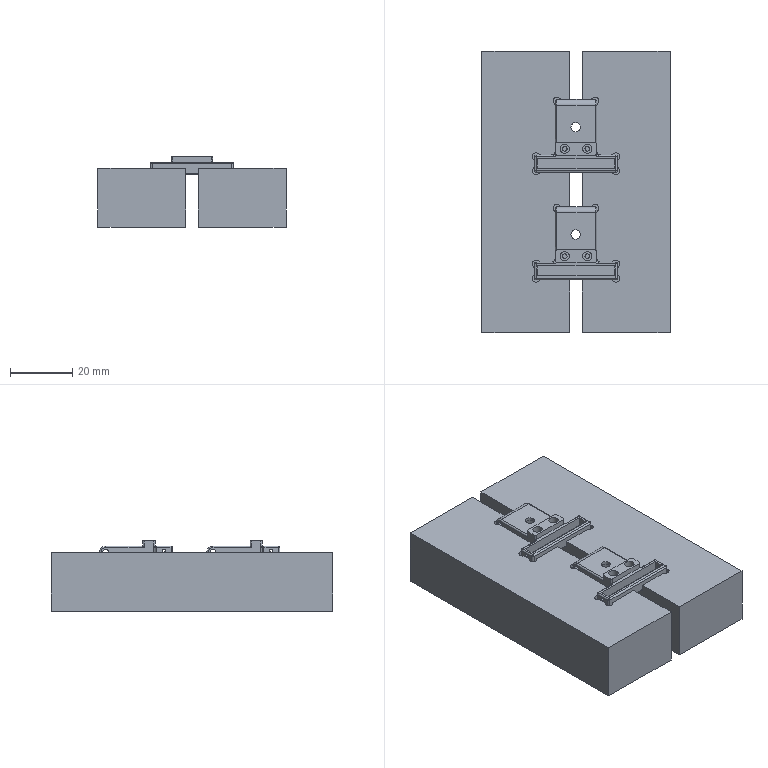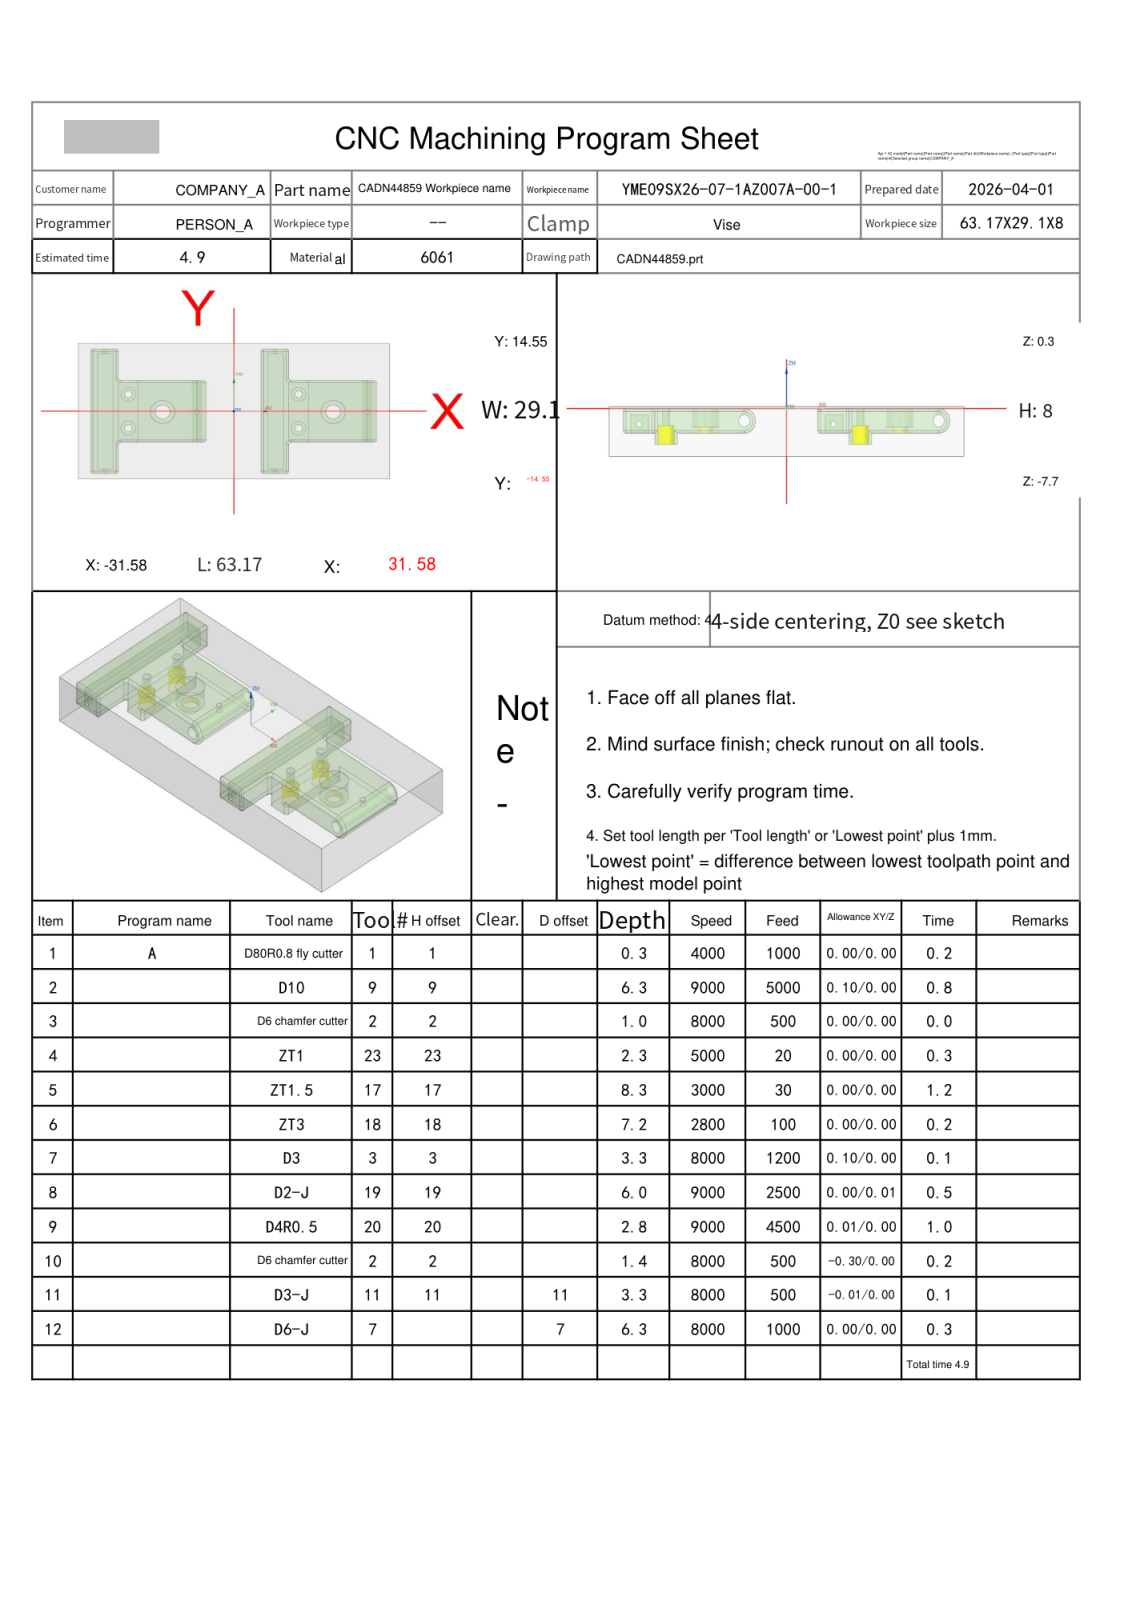NC program | NX | posted by the shop | part box 60.696 x 90.669 x 22.754 mm
Lines 834 to 2494 of 3978, first 1575 of 1661 lines:
N8 T19 M06
(D2-J  D=2. R=0. H=19 ce=0.00 di=0.01)
G00 G90 G54 X12.454 Y11.888 M03 S9000
G43 H19 Z20.
M08
Z.179
G01 X12.449 Y11.887 Z.124 F2000.
X12.435 Y11.884 Z.071
X12.414 Y11.879 Z.021
X12.386 Y11.871 Z-.027
X12.354 Y11.862 Z-.072
X12.319 Y11.849 Z-.113
X12.282 Y11.834 Z-.151
X12.245 Y11.817 Z-.185
X12.208 Y11.797 Z-.215
X12.174 Y11.774 Z-.24
X12.144 Y11.748 Z-.261
X12.12 Y11.719 Z-.276
X12.102 Y11.687 Z-.285
Y7.588 F2500.
X16.201
X16.215 Y7.603
X16.204 Y7.648 Z-.284
X16.17 Y7.719
X16.115 Y7.813 Z-.283
X15.9 Y8.13 Z-.284
X15.679 Y8.425 Z-.288
X15.384 Y8.799 Z-.299
X14.873 Y9.393 Z-.33
X14.412 Y9.885 Z-.369
X13.932 Y10.36 Z-.413
X13.348 Y10.887 Z-.468
X12.979 Y11.191 Z-.5
X12.687 Y11.419 Z-.526
X12.373 Y11.642 Z-.552
X12.279 Y11.7 Z-.56
X12.208 Y11.735 Z-.566
X12.163 Y11.747 Z-.569
X12.148 Y11.733 Z-.57
Y7.634
X16.247
X16.261 Y7.649 Z-.571
X16.25 Y7.694 Z-.574
X16.215 Y7.766 Z-.578
X16.159 Y7.861 Z-.583
X15.941 Y8.178 Z-.601
X15.718 Y8.473 Z-.619
X15.419 Y8.846 Z-.642
X14.902 Y9.435 Z-.68
X14.435 Y9.921 Z-.713
X13.949 Y10.388 Z-.746
X13.36 Y10.905 Z-.784
X12.987 Y11.204 Z-.807
X12.692 Y11.427 Z-.825
X12.375 Y11.646 Z-.843
X12.28 Y11.701 Z-.848
X12.208 Y11.736 Z-.852
X12.163 Y11.747 Z-.855
X12.148 Y11.733 Z-.856
Y7.634
X16.247
X16.261 Y7.649
X16.25 Y7.694 Z-.859
X16.215 Y7.766 Z-.863
X16.159 Y7.861 Z-.868
X15.941 Y8.178 Z-.887
X15.718 Y8.473 Z-.904
X15.419 Y8.846 Z-.927
X14.902 Y9.435 Z-.965
X14.435 Y9.921 Z-.998
X13.949 Y10.388 Z-1.031
X13.36 Y10.905 Z-1.07
X12.987 Y11.204 Z-1.092
X12.692 Y11.427 Z-1.11
X12.375 Y11.646 Z-1.128
X12.28 Y11.701 Z-1.133
X12.208 Y11.736 Z-1.137
X12.163 Y11.747 Z-1.14
X12.148 Y11.733 Z-1.141
Y7.634
X16.247
X16.261 Y7.649 Z-1.142
X16.25 Y7.694 Z-1.144
X16.215 Y7.766 Z-1.148
X16.159 Y7.861 Z-1.154
X15.941 Y8.178 Z-1.172
X15.718 Y8.473 Z-1.189
X15.419 Y8.846 Z-1.212
X14.902 Y9.435 Z-1.25
X14.435 Y9.921 Z-1.283
X13.949 Y10.388 Z-1.317
X13.36 Y10.905 Z-1.355
X12.987 Y11.204 Z-1.378
X12.692 Y11.427 Z-1.395
X12.375 Y11.646 Z-1.413
X12.28 Y11.701 Z-1.419
X12.208 Y11.736 Z-1.423
X12.163 Y11.747 Z-1.425
X12.148 Y11.733 Z-1.426
Y7.634
X16.247
X16.261 Y7.649 Z-1.427
X16.25 Y7.694 Z-1.429
X16.215 Y7.766 Z-1.433
X16.159 Y7.861 Z-1.439
X15.941 Y8.178 Z-1.457
X15.718 Y8.473 Z-1.475
X15.419 Y8.846 Z-1.497
X14.902 Y9.435 Z-1.535
X14.435 Y9.921 Z-1.569
X13.949 Y10.388 Z-1.602
X13.36 Y10.905 Z-1.64
X12.987 Y11.204 Z-1.663
X12.692 Y11.427 Z-1.68
X12.375 Y11.646 Z-1.698
X12.28 Y11.701 Z-1.704
X12.208 Y11.736 Z-1.708
X12.163 Y11.747 Z-1.71
X12.148 Y11.733 Z-1.711
Y7.634
X16.247
X16.261 Y7.649 Z-1.712
X16.25 Y7.694 Z-1.715
X16.215 Y7.766 Z-1.719
X16.159 Y7.861 Z-1.724
X15.941 Y8.178 Z-1.742
X15.718 Y8.473 Z-1.76
X15.419 Y8.846 Z-1.782
X14.902 Y9.435 Z-1.821
X14.435 Y9.921 Z-1.854
X13.949 Y10.388 Z-1.887
X13.36 Y10.905 Z-1.925
X12.987 Y11.204 Z-1.948
X12.692 Y11.427 Z-1.965
X12.375 Y11.646 Z-1.984
X12.28 Y11.701 Z-1.989
X12.208 Y11.736 Z-1.993
X12.163 Y11.747 Z-1.996
X12.148 Y11.733
Y7.634
X16.247
X16.261 Y7.649 Z-1.997
X16.25 Y7.694 Z-2.
X16.215 Y7.766 Z-2.004
X16.159 Y7.861 Z-2.009
X15.941 Y8.178 Z-2.027
X15.718 Y8.473 Z-2.045
X15.419 Y8.846 Z-2.068
X14.902 Y9.436 Z-2.106
X14.435 Y9.921 Z-2.139
X13.949 Y10.388 Z-2.172
X13.36 Y10.905 Z-2.21
X12.987 Y11.204 Z-2.233
X12.692 Y11.427 Z-2.251
X12.375 Y11.646 Z-2.269
X12.28 Y11.701 Z-2.274
X12.208 Y11.736 Z-2.278
X12.163 Y11.747 Z-2.281
X12.148 Y11.733 Z-2.282
Y7.634
X16.247
X16.261 Y7.649
X16.25 Y7.694 Z-2.285
X16.215 Y7.766 Z-2.289
X16.159 Y7.861 Z-2.294
X15.941 Y8.178 Z-2.313
X15.718 Y8.473 Z-2.33
X15.419 Y8.846 Z-2.353
X14.902 Y9.436 Z-2.391
X14.435 Y9.921 Z-2.424
X13.949 Y10.388 Z-2.457
X13.36 Y10.905 Z-2.496
X12.987 Y11.204 Z-2.518
X12.692 Y11.427 Z-2.536
X12.375 Y11.646 Z-2.554
X12.28 Y11.701 Z-2.559
X12.208 Y11.736 Z-2.563
X12.163 Y11.747 Z-2.566
X12.148 Y11.733 Z-2.567
Y7.634
X16.247
X16.261 Y7.649 Z-2.568
X16.25 Y7.694 Z-2.57
X16.215 Y7.766 Z-2.574
X16.159 Y7.861 Z-2.58
X15.941 Y8.178 Z-2.598
X15.718 Y8.473 Z-2.615
X15.419 Y8.846 Z-2.638
X14.902 Y9.436 Z-2.676
X14.435 Y9.921 Z-2.709
X13.949 Y10.388 Z-2.743
X13.36 Y10.905 Z-2.781
X12.987 Y11.204 Z-2.804
X12.692 Y11.427 Z-2.821
X12.375 Y11.646 Z-2.839
X12.28 Y11.701 Z-2.845
X12.208 Y11.736 Z-2.849
X12.163 Y11.747 Z-2.851
X12.148 Y11.733 Z-2.852
Y7.634
X16.247
X16.261 Y7.649 Z-2.853
X16.25 Y7.694 Z-2.855
X16.215 Y7.766 Z-2.859
X16.159 Y7.861 Z-2.865
X15.941 Y8.178 Z-2.883
X15.718 Y8.473 Z-2.901
X15.419 Y8.846 Z-2.923
X14.902 Y9.436 Z-2.961
X14.435 Y9.921 Z-2.995
X13.949 Y10.388 Z-3.028
X13.36 Y10.905 Z-3.066
X12.987 Y11.204 Z-3.089
X12.692 Y11.427 Z-3.106
X12.375 Y11.646 Z-3.125
X12.28 Y11.701 Z-3.13
X12.208 Y11.736 Z-3.134
X12.163 Y11.747 Z-3.136
X12.148 Y11.733 Z-3.137
Y7.634
X16.247
X16.261 Y7.649 Z-3.138
X16.25 Y7.694 Z-3.141
X16.215 Y7.766 Z-3.145
X16.159 Y7.861 Z-3.15
X15.941 Y8.178 Z-3.168
X15.718 Y8.473 Z-3.186
X15.419 Y8.846 Z-3.208
X14.902 Y9.436 Z-3.247
X14.435 Y9.921 Z-3.28
X13.949 Y10.388 Z-3.313
X13.36 Y10.905 Z-3.351
X12.987 Y11.204 Z-3.374
X12.692 Y11.427 Z-3.391
X12.375 Y11.646 Z-3.41
X12.28 Y11.701 Z-3.415
X12.208 Y11.736 Z-3.419
X12.163 Y11.747 Z-3.422
X12.148 Y11.733
Y7.634
X16.247
X16.261 Y7.649 Z-3.423
X16.25 Y7.694 Z-3.426
X16.215 Y7.766 Z-3.43
X16.159 Y7.861 Z-3.435
X15.941 Y8.178 Z-3.453
X15.718 Y8.474 Z-3.471
X15.419 Y8.847 Z-3.494
X14.902 Y9.437 Z-3.532
X14.435 Y9.923 Z-3.565
X13.949 Y10.39 Z-3.598
X13.36 Y10.907 Z-3.636
X12.987 Y11.207 Z-3.659
X12.692 Y11.43 Z-3.677
X12.375 Y11.649 Z-3.695
X12.28 Y11.705 Z-3.7
X12.208 Y11.739 Z-3.704
X12.163 Y11.751 Z-3.707
X12.148 Y11.737 Z-3.708
Y7.634
X16.249
X16.263 Y7.649
X16.252 Y7.694 Z-3.711
X16.217 Y7.766 Z-3.715
X16.161 Y7.861 Z-3.72
X15.943 Y8.178 Z-3.739
X15.72 Y8.474 Z-3.756
X15.42 Y8.847 Z-3.779
X14.903 Y9.437 Z-3.817
X14.436 Y9.923 Z-3.85
X13.95 Y10.39 Z-3.883
X13.36 Y10.907 Z-3.922
X12.987 Y11.207 Z-3.944
X12.692 Y11.43 Z-3.962
X12.375 Y11.649 Z-3.98
X12.28 Y11.705 Z-3.985
X12.208 Y11.739 Z-3.989
X12.163 Y11.751 Z-3.992
X12.148 Y11.737 Z-3.993
Y7.634
X16.249
X16.263 Y7.649 Z-3.994
X16.252 Y7.694 Z-3.996
X16.217 Y7.766 Z-4.
X16.161 Y7.861 Z-4.006
X15.943 Y8.178 Z-4.024
X15.72 Y8.474 Z-4.041
X15.42 Y8.847 Z-4.064
X14.903 Y9.437 Z-4.102
X14.436 Y9.923 Z-4.135
X13.95 Y10.39 Z-4.169
X13.36 Y10.907 Z-4.207
X12.987 Y11.207 Z-4.23
X12.692 Y11.43 Z-4.247
X12.375 Y11.649 Z-4.265
X12.28 Y11.705 Z-4.271
X12.208 Y11.739 Z-4.275
X12.163 Y11.751 Z-4.277
X12.148 Y11.737 Z-4.278
Y7.634
X16.249
X16.263 Y7.649 Z-4.279
X16.252 Y7.694 Z-4.281
X16.217 Y7.766 Z-4.285
X16.161 Y7.861 Z-4.291
X15.943 Y8.178 Z-4.309
X15.72 Y8.474 Z-4.327
X15.42 Y8.847 Z-4.349
X14.903 Y9.437 Z-4.387
X14.436 Y9.923 Z-4.421
X13.95 Y10.39 Z-4.454
X13.36 Y10.907 Z-4.492
X12.987 Y11.207 Z-4.515
X12.692 Y11.43 Z-4.532
X12.375 Y11.649 Z-4.551
X12.28 Y11.705 Z-4.556
X12.208 Y11.739 Z-4.56
X12.163 Y11.751 Z-4.562
X12.148 Y11.737 Z-4.563
Y7.634
X16.249
X16.263 Y7.649 Z-4.564
X16.252 Y7.694 Z-4.567
X16.217 Y7.766 Z-4.571
X16.161 Y7.861 Z-4.576
X15.943 Y8.178 Z-4.594
X15.72 Y8.474 Z-4.612
X15.42 Y8.847 Z-4.634
X14.903 Y9.437 Z-4.673
X14.436 Y9.923 Z-4.706
X13.95 Y10.39 Z-4.739
X13.36 Y10.907 Z-4.777
X12.987 Y11.207 Z-4.8
X12.692 Y11.43 Z-4.817
X12.375 Y11.649 Z-4.836
X12.28 Y11.705 Z-4.841
X12.208 Y11.739 Z-4.845
X12.163 Y11.751 Z-4.848
X12.148 Y11.737
Y7.634
X16.249
X16.263 Y7.649 Z-4.849
X16.252 Y7.694 Z-4.852
X16.217 Y7.766 Z-4.856
X16.161 Y7.861 Z-4.861
X15.943 Y8.178 Z-4.879
X15.72 Y8.474 Z-4.897
X15.42 Y8.847 Z-4.92
X14.903 Y9.437 Z-4.958
X14.436 Y9.923 Z-4.991
X13.95 Y10.39 Z-5.024
X13.36 Y10.907 Z-5.062
X12.987 Y11.207 Z-5.085
X12.692 Y11.43 Z-5.103
X12.375 Y11.649 Z-5.121
X12.28 Y11.705 Z-5.126
X12.208 Y11.739 Z-5.13
X12.163 Y11.751 Z-5.133
X12.148 Y11.737 Z-5.134
Y7.634
X16.249
X16.263 Y7.649
X16.252 Y7.694 Z-5.137
X16.217 Y7.766 Z-5.141
X16.161 Y7.861 Z-5.146
X15.943 Y8.178 Z-5.165
X15.72 Y8.474 Z-5.182
X15.42 Y8.847 Z-5.205
X14.903 Y9.437 Z-5.243
X14.436 Y9.923 Z-5.276
X13.95 Y10.39 Z-5.309
X13.36 Y10.907 Z-5.348
X12.987 Y11.207 Z-5.37
X12.692 Y11.43 Z-5.388
X12.375 Y11.649 Z-5.406
X12.28 Y11.705 Z-5.411
X12.208 Y11.739 Z-5.415
X12.163 Y11.751 Z-5.418
X12.148 Y11.737 Z-5.419
Y7.634
X16.249
X16.263 Y7.649 Z-5.42
X16.252 Y7.694 Z-5.422
X16.217 Y7.766 Z-5.426
X16.161 Y7.861 Z-5.432
X15.943 Y8.178 Z-5.45
X15.72 Y8.474 Z-5.467
X15.42 Y8.847 Z-5.49
X14.903 Y9.437 Z-5.528
X14.436 Y9.923 Z-5.561
X13.95 Y10.39 Z-5.595
X13.36 Y10.907 Z-5.633
X12.987 Y11.207 Z-5.656
X12.692 Y11.43 Z-5.673
X12.375 Y11.649 Z-5.691
X12.28 Y11.705 Z-5.697
X12.208 Y11.739 Z-5.701
X12.163 Y11.751 Z-5.703
X12.148 Y11.737 Z-5.704
Y7.634
X16.249
X16.363 Y7.643 Z-5.702
X16.466 Y7.67 Z-5.695
X16.558 Y7.712 Z-5.684
X16.639 Y7.765 Z-5.666
X16.71 Y7.828 Z-5.643
X16.772 Y7.898 Z-5.613
X16.826 Y7.972 Z-5.576
X16.871 Y8.047 Z-5.531
X16.908 Y8.12 Z-5.477
X16.938 Y8.19 Z-5.415
X16.961 Y8.253 Z-5.344
X16.979 Y8.306 Z-5.262
X16.99 Y8.348 Z-5.171
X16.997 Y8.375 Z-5.068
X16.999 Y8.384 Z-4.954
G00 Z20.
X16.382 Y-7.937
Z.176
G01 Y-7.932 Z.122 F2000.
X16.379 Y-7.918 Z.069
X16.376 Y-7.897 Z.019
X16.37 Y-7.87 Z-.029
X16.362 Y-7.838 Z-.073
X16.352 Y-7.803 Z-.115
X16.339 Y-7.767 Z-.152
X16.324 Y-7.73 Z-.186
X16.306 Y-7.694 Z-.216
X16.285 Y-7.66 Z-.241
X16.261 Y-7.63 Z-.261
X16.233 Y-7.606 Z-.276
X16.201 Y-7.588 Z-.285
X12.102 F2500.
Y-11.687
X12.117 Y-11.701
X12.162 Y-11.69 Z-.284
X12.233 Y-11.657
X12.327 Y-11.602 Z-.283
X12.644 Y-11.387 Z-.284
X12.939 Y-11.167 Z-.288
X13.313 Y-10.872 Z-.298
X13.907 Y-10.362 Z-.33
X14.399 Y-9.901 Z-.369
X14.874 Y-9.421 Z-.413
X15.401 Y-8.837 Z-.467
X15.705 Y-8.468 Z-.5
X15.933 Y-8.174 Z-.526
X16.156 Y-7.859 Z-.552
X16.213 Y-7.765 Z-.56
X16.249 Y-7.694 Z-.566
X16.261 Y-7.649 Z-.569
X16.247 Y-7.634 Z-.57
X12.148
Y-11.733
X12.163 Y-11.747 Z-.571
X12.208 Y-11.736 Z-.574
X12.28 Y-11.701 Z-.578
X12.375 Y-11.646 Z-.583
X12.692 Y-11.427 Z-.601
X12.987 Y-11.204 Z-.619
X13.36 Y-10.905 Z-.642
X13.949 Y-10.389 Z-.68
X14.435 Y-9.922 Z-.713
X14.902 Y-9.436 Z-.746
X15.419 Y-8.846 Z-.784
X15.718 Y-8.474 Z-.807
X15.941 Y-8.178 Z-.825
X16.159 Y-7.861 Z-.843
X16.215 Y-7.766 Z-.848
X16.25 Y-7.694 Z-.852
X16.261 Y-7.649 Z-.855
X16.247 Y-7.634 Z-.856
X12.148
Y-11.733
X12.163 Y-11.747
X12.208 Y-11.736 Z-.859
X12.28 Y-11.701 Z-.863
X12.375 Y-11.646 Z-.868
X12.692 Y-11.427 Z-.887
X12.987 Y-11.204 Z-.904
X13.36 Y-10.905 Z-.927
X13.949 Y-10.388 Z-.965
X14.435 Y-9.922 Z-.998
X14.902 Y-9.436 Z-1.031
X15.419 Y-8.846 Z-1.07
X15.718 Y-8.474 Z-1.092
X15.941 Y-8.178 Z-1.11
X16.159 Y-7.861 Z-1.128
X16.215 Y-7.766 Z-1.133
X16.25 Y-7.694 Z-1.137
X16.261 Y-7.649 Z-1.14
X16.247 Y-7.634 Z-1.141
X12.148
Y-11.733
X12.163 Y-11.747 Z-1.142
X12.208 Y-11.736 Z-1.144
X12.28 Y-11.701 Z-1.148
X12.375 Y-11.646 Z-1.154
X12.692 Y-11.427 Z-1.172
X12.987 Y-11.204 Z-1.189
X13.36 Y-10.905 Z-1.212
X13.949 Y-10.388 Z-1.25
X14.435 Y-9.922 Z-1.283
X14.902 Y-9.436 Z-1.317
X15.419 Y-8.846 Z-1.355
X15.718 Y-8.474 Z-1.378
X15.941 Y-8.178 Z-1.395
X16.159 Y-7.861 Z-1.413
X16.215 Y-7.766 Z-1.419
X16.25 Y-7.694 Z-1.423
X16.261 Y-7.649 Z-1.425
X16.247 Y-7.634 Z-1.426
X12.148
Y-11.733
X12.163 Y-11.747 Z-1.427
X12.208 Y-11.736 Z-1.429
X12.28 Y-11.701 Z-1.433
X12.375 Y-11.646 Z-1.439
X12.692 Y-11.427 Z-1.457
X12.987 Y-11.204 Z-1.475
X13.36 Y-10.905 Z-1.497
X13.949 Y-10.388 Z-1.535
X14.435 Y-9.921 Z-1.569
X14.902 Y-9.436 Z-1.602
X15.419 Y-8.846 Z-1.64
X15.718 Y-8.473 Z-1.663
X15.941 Y-8.178 Z-1.68
X16.159 Y-7.861 Z-1.698
X16.215 Y-7.766 Z-1.704
X16.25 Y-7.694 Z-1.708
X16.261 Y-7.649 Z-1.71
X16.247 Y-7.634 Z-1.711
X12.148
Y-11.733
X12.163 Y-11.747 Z-1.712
X12.208 Y-11.736 Z-1.715
X12.28 Y-11.701 Z-1.719
X12.375 Y-11.646 Z-1.724
X12.692 Y-11.427 Z-1.742
X12.987 Y-11.204 Z-1.76
X13.36 Y-10.905 Z-1.782
X13.949 Y-10.388 Z-1.821
X14.435 Y-9.922 Z-1.854
X14.902 Y-9.436 Z-1.887
X15.419 Y-8.846 Z-1.925
X15.718 Y-8.474 Z-1.948
X15.941 Y-8.178 Z-1.965
X16.159 Y-7.861 Z-1.984
X16.215 Y-7.766 Z-1.989
X16.25 Y-7.694 Z-1.993
X16.261 Y-7.649 Z-1.996
X16.247 Y-7.634
X12.148
Y-11.733
X12.163 Y-11.747 Z-1.997
X12.208 Y-11.736 Z-2.
X12.28 Y-11.701 Z-2.004
X12.375 Y-11.646 Z-2.009
X12.692 Y-11.427 Z-2.027
X12.987 Y-11.204 Z-2.045
X13.36 Y-10.905 Z-2.068
X13.949 Y-10.388 Z-2.106
X14.435 Y-9.921 Z-2.139
X14.902 Y-9.436 Z-2.172
X15.419 Y-8.846 Z-2.21
X15.718 Y-8.473 Z-2.233
X15.941 Y-8.178 Z-2.251
X16.159 Y-7.861 Z-2.269
X16.215 Y-7.766 Z-2.274
X16.25 Y-7.694 Z-2.278
X16.261 Y-7.649 Z-2.281
X16.247 Y-7.634 Z-2.282
X12.148
Y-11.733
X12.163 Y-11.747
X12.208 Y-11.736 Z-2.285
X12.28 Y-11.701 Z-2.289
X12.375 Y-11.646 Z-2.294
X12.692 Y-11.427 Z-2.313
X12.987 Y-11.204 Z-2.33
X13.36 Y-10.905 Z-2.353
X13.949 Y-10.388 Z-2.391
X14.435 Y-9.921 Z-2.424
X14.902 Y-9.436 Z-2.457
X15.419 Y-8.846 Z-2.496
X15.718 Y-8.473 Z-2.518
X15.941 Y-8.178 Z-2.536
X16.159 Y-7.861 Z-2.554
X16.215 Y-7.766 Z-2.559
X16.25 Y-7.694 Z-2.563
X16.261 Y-7.649 Z-2.566
X16.247 Y-7.634 Z-2.567
X12.148
Y-11.733
X12.163 Y-11.747 Z-2.568
X12.208 Y-11.736 Z-2.57
X12.28 Y-11.701 Z-2.574
X12.375 Y-11.646 Z-2.58
X12.692 Y-11.427 Z-2.598
X12.987 Y-11.204 Z-2.615
X13.36 Y-10.905 Z-2.638
X13.949 Y-10.388 Z-2.676
X14.435 Y-9.921 Z-2.709
X14.902 Y-9.436 Z-2.743
X15.419 Y-8.846 Z-2.781
X15.718 Y-8.473 Z-2.804
X15.941 Y-8.178 Z-2.821
X16.159 Y-7.861 Z-2.839
X16.215 Y-7.766 Z-2.845
X16.25 Y-7.694 Z-2.849
X16.261 Y-7.649 Z-2.851
X16.247 Y-7.634 Z-2.852
X12.148
Y-11.733
X12.163 Y-11.747 Z-2.853
X12.208 Y-11.736 Z-2.855
X12.28 Y-11.701 Z-2.859
X12.375 Y-11.646 Z-2.865
X12.692 Y-11.427 Z-2.883
X12.987 Y-11.204 Z-2.901
X13.36 Y-10.905 Z-2.923
X13.949 Y-10.388 Z-2.961
X14.435 Y-9.921 Z-2.995
X14.902 Y-9.436 Z-3.028
X15.419 Y-8.846 Z-3.066
X15.718 Y-8.473 Z-3.089
X15.941 Y-8.178 Z-3.106
X16.159 Y-7.861 Z-3.125
X16.215 Y-7.766 Z-3.13
X16.25 Y-7.694 Z-3.134
X16.261 Y-7.649 Z-3.136
X16.247 Y-7.634 Z-3.137
X12.148
Y-11.733
X12.163 Y-11.747 Z-3.138
X12.208 Y-11.736 Z-3.141
X12.28 Y-11.701 Z-3.145
X12.375 Y-11.646 Z-3.15
X12.692 Y-11.427 Z-3.168
X12.987 Y-11.204 Z-3.186
X13.36 Y-10.905 Z-3.208
X13.949 Y-10.388 Z-3.247
X14.435 Y-9.921 Z-3.28
X14.902 Y-9.436 Z-3.313
X15.419 Y-8.846 Z-3.351
X15.718 Y-8.473 Z-3.374
X15.941 Y-8.178 Z-3.391
X16.159 Y-7.861 Z-3.41
X16.215 Y-7.766 Z-3.415
X16.25 Y-7.694 Z-3.419
X16.261 Y-7.649 Z-3.422
X16.247 Y-7.634
X12.148
Y-11.733
X12.163 Y-11.747 Z-3.423
X12.208 Y-11.736 Z-3.426
X12.28 Y-11.701 Z-3.43
X12.375 Y-11.646 Z-3.435
X12.692 Y-11.427 Z-3.453
X12.987 Y-11.204 Z-3.471
X13.36 Y-10.905 Z-3.494
X13.95 Y-10.388 Z-3.532
X14.436 Y-9.921 Z-3.565
X14.903 Y-9.436 Z-3.598
X15.42 Y-8.846 Z-3.636
X15.72 Y-8.473 Z-3.659
X15.943 Y-8.178 Z-3.677
X16.161 Y-7.861 Z-3.695
X16.217 Y-7.766 Z-3.7
X16.252 Y-7.694 Z-3.704
X16.263 Y-7.649 Z-3.707
X16.249 Y-7.634 Z-3.708
X12.148
Y-11.737
X12.163 Y-11.751
X12.208 Y-11.739 Z-3.711
X12.28 Y-11.705 Z-3.715
X12.375 Y-11.649 Z-3.72
X12.692 Y-11.43 Z-3.739
X12.987 Y-11.207 Z-3.756
X13.36 Y-10.908 Z-3.779
X13.95 Y-10.39 Z-3.817
X14.436 Y-9.923 Z-3.85
X14.903 Y-9.437 Z-3.883
X15.42 Y-8.847 Z-3.922
X15.72 Y-8.474 Z-3.944
X15.943 Y-8.178 Z-3.962
X16.161 Y-7.861 Z-3.98
X16.217 Y-7.766 Z-3.985
X16.252 Y-7.694 Z-3.989
X16.263 Y-7.649 Z-3.992
X16.249 Y-7.634 Z-3.993
X12.148
Y-11.737
X12.163 Y-11.751 Z-3.994
X12.208 Y-11.739 Z-3.996
X12.28 Y-11.705 Z-4.
X12.375 Y-11.649 Z-4.006
X12.692 Y-11.43 Z-4.024
X12.987 Y-11.207 Z-4.041
X13.36 Y-10.908 Z-4.064
X13.95 Y-10.39 Z-4.102
X14.436 Y-9.923 Z-4.135
X14.903 Y-9.437 Z-4.169
X15.42 Y-8.847 Z-4.207
X15.72 Y-8.474 Z-4.23
X15.943 Y-8.178 Z-4.247
X16.161 Y-7.861 Z-4.265
X16.217 Y-7.766 Z-4.271
X16.252 Y-7.694 Z-4.275
X16.263 Y-7.649 Z-4.277
X16.249 Y-7.634 Z-4.278
X12.148
Y-11.737
X12.163 Y-11.751 Z-4.279
X12.208 Y-11.739 Z-4.281
X12.28 Y-11.705 Z-4.285
X12.375 Y-11.649 Z-4.291
X12.692 Y-11.43 Z-4.309
X12.987 Y-11.207 Z-4.327
X13.36 Y-10.908 Z-4.349
X13.95 Y-10.39 Z-4.387
X14.436 Y-9.923 Z-4.421
X14.903 Y-9.437 Z-4.454
X15.42 Y-8.847 Z-4.492
X15.72 Y-8.474 Z-4.515
X15.943 Y-8.178 Z-4.532
X16.161 Y-7.861 Z-4.551
X16.217 Y-7.766 Z-4.556
X16.252 Y-7.694 Z-4.56
X16.263 Y-7.649 Z-4.562
X16.249 Y-7.634 Z-4.563
X12.148
Y-11.737
X12.163 Y-11.751 Z-4.564
X12.208 Y-11.739 Z-4.567
X12.28 Y-11.705 Z-4.571
X12.375 Y-11.649 Z-4.576
X12.692 Y-11.43 Z-4.594
X12.987 Y-11.207 Z-4.612
X13.36 Y-10.908 Z-4.634
X13.95 Y-10.39 Z-4.673
X14.436 Y-9.923 Z-4.706
X14.903 Y-9.437 Z-4.739
X15.42 Y-8.847 Z-4.777
X15.72 Y-8.474 Z-4.8
X15.943 Y-8.178 Z-4.817
X16.161 Y-7.861 Z-4.836
X16.217 Y-7.766 Z-4.841
X16.252 Y-7.694 Z-4.845
X16.263 Y-7.649 Z-4.848
X16.249 Y-7.634
X12.148
Y-11.737
X12.163 Y-11.751 Z-4.849
X12.208 Y-11.739 Z-4.852
X12.28 Y-11.705 Z-4.856
X12.375 Y-11.649 Z-4.861
X12.692 Y-11.43 Z-4.879
X12.987 Y-11.207 Z-4.897
X13.36 Y-10.908 Z-4.92
X13.95 Y-10.39 Z-4.958
X14.436 Y-9.923 Z-4.991
X14.903 Y-9.437 Z-5.024
X15.42 Y-8.847 Z-5.062
X15.72 Y-8.474 Z-5.085
X15.943 Y-8.178 Z-5.103
X16.161 Y-7.861 Z-5.121
X16.217 Y-7.766 Z-5.126
X16.252 Y-7.694 Z-5.13
X16.263 Y-7.649 Z-5.133
X16.249 Y-7.634 Z-5.134
X12.148
Y-11.737
X12.163 Y-11.751
X12.208 Y-11.739 Z-5.137
X12.28 Y-11.705 Z-5.141
X12.375 Y-11.649 Z-5.146
X12.692 Y-11.43 Z-5.165
X12.987 Y-11.207 Z-5.182
X13.36 Y-10.908 Z-5.205
X13.95 Y-10.39 Z-5.243
X14.436 Y-9.923 Z-5.276
X14.903 Y-9.437 Z-5.309
X15.42 Y-8.847 Z-5.348
X15.72 Y-8.474 Z-5.37
X15.943 Y-8.178 Z-5.388
X16.161 Y-7.861 Z-5.406
X16.217 Y-7.766 Z-5.411
X16.252 Y-7.694 Z-5.415
X16.263 Y-7.649 Z-5.418
X16.249 Y-7.634 Z-5.419
X12.148
Y-11.737
X12.163 Y-11.751 Z-5.42
X12.208 Y-11.739 Z-5.422
X12.28 Y-11.705 Z-5.426
X12.375 Y-11.649 Z-5.432
X12.692 Y-11.43 Z-5.45
X12.987 Y-11.207 Z-5.467
X13.36 Y-10.908 Z-5.49
X13.95 Y-10.39 Z-5.528
X14.436 Y-9.923 Z-5.561
X14.903 Y-9.437 Z-5.595
X15.42 Y-8.847 Z-5.633
X15.72 Y-8.474 Z-5.656
X15.943 Y-8.178 Z-5.673
X16.161 Y-7.861 Z-5.691
X16.217 Y-7.766 Z-5.697
X16.252 Y-7.694 Z-5.701
X16.263 Y-7.649 Z-5.703
X16.249 Y-7.634 Z-5.704
X12.148
Y-11.737
X12.157 Y-11.851 Z-5.702
X12.184 Y-11.953 Z-5.695
X12.226 Y-12.045 Z-5.684
X12.279 Y-12.126 Z-5.666
X12.342 Y-12.198 Z-5.643
X12.412 Y-12.26 Z-5.613
X12.485 Y-12.313 Z-5.576
X12.56 Y-12.358 Z-5.531
X12.634 Y-12.395 Z-5.477
X12.703 Y-12.425 Z-5.415
X12.766 Y-12.449 Z-5.344
X12.82 Y-12.466 Z-5.262
X12.861 Y-12.478 Z-5.171
X12.888 Y-12.484 Z-5.068
X12.898 Y-12.487 Z-4.954
G00 Z20.
X-22.146 Y11.888
Z.179
G01 X-22.151 Y11.887 Z.124 F2000.
X-22.165 Y11.884 Z.072
X-22.187 Y11.879 Z.021
X-22.214 Y11.871 Z-.027
X-22.246 Y11.862 Z-.071
X-22.281 Y11.849 Z-.113
X-22.318 Y11.834 Z-.151
X-22.355 Y11.817 Z-.185
X-22.392 Y11.797 Z-.215
X-22.426 Y11.774 Z-.24
X-22.456 Y11.748 Z-.261
X-22.48 Y11.719 Z-.276
X-22.498 Y11.687 Z-.285
Y7.588 F2500.
X-18.399
X-18.385 Y7.603
X-18.396 Y7.648 Z-.284
X-18.43 Y7.719
X-18.485 Y7.813 Z-.283
X-18.7 Y8.13 Z-.284
X-18.921 Y8.425 Z-.288
X-19.216 Y8.799 Z-.299
X-19.727 Y9.393 Z-.33
X-20.188 Y9.885 Z-.369
X-20.668 Y10.36 Z-.413
X-21.252 Y10.887 Z-.468
X-21.621 Y11.191 Z-.5
X-21.913 Y11.419 Z-.526
X-22.227 Y11.642 Z-.552
X-22.321 Y11.7 Z-.56
X-22.392 Y11.735 Z-.566
X-22.437 Y11.747 Z-.569
X-22.452 Y11.733 Z-.57
Y7.634
X-18.353
X-18.339 Y7.649 Z-.571
X-18.35 Y7.694 Z-.574
X-18.385 Y7.766 Z-.578
X-18.441 Y7.861 Z-.583
X-18.659 Y8.178 Z-.601
X-18.882 Y8.473 Z-.619
X-19.181 Y8.846 Z-.642
X-19.698 Y9.435 Z-.68
X-20.165 Y9.921 Z-.713
X-20.651 Y10.388 Z-.746
X-21.24 Y10.905 Z-.784
X-21.613 Y11.204 Z-.807
X-21.908 Y11.427 Z-.825
X-22.225 Y11.646 Z-.843
X-22.32 Y11.701 Z-.848
X-22.392 Y11.736 Z-.852
X-22.437 Y11.747 Z-.855
X-22.452 Y11.733 Z-.856
Y7.634
X-18.353
X-18.339 Y7.649
X-18.35 Y7.694 Z-.859
X-18.385 Y7.766 Z-.863
X-18.441 Y7.861 Z-.868
X-18.659 Y8.178 Z-.887
X-18.882 Y8.473 Z-.904
X-19.181 Y8.846 Z-.927
X-19.698 Y9.435 Z-.965
X-20.165 Y9.921 Z-.998
X-20.651 Y10.388 Z-1.031
X-21.24 Y10.905 Z-1.07
X-21.613 Y11.204 Z-1.092
X-21.908 Y11.427 Z-1.11
X-22.225 Y11.646 Z-1.128
X-22.32 Y11.701 Z-1.133
X-22.392 Y11.736 Z-1.137
X-22.437 Y11.747 Z-1.14
X-22.452 Y11.733 Z-1.141
Y7.634
X-18.353
X-18.339 Y7.649 Z-1.142
X-18.35 Y7.694 Z-1.144
X-18.385 Y7.766 Z-1.148
X-18.441 Y7.861 Z-1.154
X-18.659 Y8.178 Z-1.172
X-18.882 Y8.473 Z-1.189
X-19.181 Y8.846 Z-1.212
X-19.698 Y9.435 Z-1.25
X-20.165 Y9.921 Z-1.283
X-20.651 Y10.388 Z-1.317
X-21.24 Y10.905 Z-1.355
X-21.613 Y11.204 Z-1.378
X-21.908 Y11.427 Z-1.395
X-22.225 Y11.646 Z-1.413
X-22.32 Y11.701 Z-1.419
X-22.392 Y11.736 Z-1.423
X-22.437 Y11.747 Z-1.425
X-22.452 Y11.733 Z-1.426
Y7.634
X-18.353
X-18.339 Y7.649 Z-1.427
X-18.35 Y7.694 Z-1.429
X-18.385 Y7.766 Z-1.433
X-18.441 Y7.861 Z-1.439
X-18.659 Y8.178 Z-1.457
X-18.882 Y8.473 Z-1.475
X-19.181 Y8.846 Z-1.497
X-19.698 Y9.435 Z-1.535
X-20.165 Y9.921 Z-1.569
X-20.651 Y10.388 Z-1.602
X-21.24 Y10.905 Z-1.64
X-21.613 Y11.204 Z-1.663
X-21.908 Y11.427 Z-1.68
X-22.225 Y11.646 Z-1.698
X-22.32 Y11.701 Z-1.704
X-22.392 Y11.736 Z-1.708
X-22.437 Y11.747 Z-1.71
X-22.452 Y11.733 Z-1.711
Y7.634
X-18.353
X-18.339 Y7.649 Z-1.712
X-18.35 Y7.694 Z-1.715
X-18.385 Y7.766 Z-1.719
X-18.441 Y7.861 Z-1.724
X-18.659 Y8.178 Z-1.742
X-18.882 Y8.473 Z-1.76
X-19.181 Y8.846 Z-1.782
X-19.698 Y9.435 Z-1.821
X-20.165 Y9.921 Z-1.854
X-20.651 Y10.388 Z-1.887
X-21.24 Y10.905 Z-1.925
X-21.613 Y11.204 Z-1.948
X-21.908 Y11.427 Z-1.965
X-22.225 Y11.646 Z-1.984
X-22.32 Y11.701 Z-1.989
X-22.392 Y11.736 Z-1.993
X-22.437 Y11.747 Z-1.996
X-22.452 Y11.733
Y7.634
X-18.353
X-18.339 Y7.649 Z-1.997
X-18.35 Y7.694 Z-2.
X-18.385 Y7.766 Z-2.004
X-18.441 Y7.861 Z-2.009
X-18.659 Y8.178 Z-2.027
X-18.882 Y8.473 Z-2.045
X-19.181 Y8.846 Z-2.068
X-19.698 Y9.436 Z-2.106
X-20.165 Y9.921 Z-2.139
X-20.651 Y10.388 Z-2.172
X-21.24 Y10.905 Z-2.21
X-21.613 Y11.204 Z-2.233
X-21.908 Y11.427 Z-2.251
X-22.225 Y11.646 Z-2.269
X-22.32 Y11.701 Z-2.274
X-22.392 Y11.736 Z-2.278
X-22.437 Y11.747 Z-2.281
X-22.452 Y11.733 Z-2.282
Y7.634
X-18.353
X-18.339 Y7.649
X-18.35 Y7.694 Z-2.285
X-18.385 Y7.766 Z-2.289
X-18.441 Y7.861 Z-2.294
X-18.659 Y8.178 Z-2.313
X-18.882 Y8.473 Z-2.33
X-19.181 Y8.846 Z-2.353
X-19.698 Y9.436 Z-2.391
X-20.165 Y9.921 Z-2.424
X-20.651 Y10.388 Z-2.457
X-21.24 Y10.905 Z-2.496
X-21.613 Y11.204 Z-2.518
X-21.908 Y11.427 Z-2.536
X-22.225 Y11.646 Z-2.554
X-22.32 Y11.701 Z-2.559
X-22.392 Y11.736 Z-2.563
X-22.437 Y11.747 Z-2.566
X-22.452 Y11.733 Z-2.567
Y7.634
X-18.353
X-18.339 Y7.649 Z-2.568
X-18.35 Y7.694 Z-2.57
X-18.385 Y7.766 Z-2.574
X-18.441 Y7.861 Z-2.58
X-18.659 Y8.178 Z-2.598
X-18.882 Y8.473 Z-2.615
X-19.181 Y8.846 Z-2.638
X-19.698 Y9.436 Z-2.676
X-20.165 Y9.921 Z-2.709
X-20.651 Y10.388 Z-2.743
X-21.24 Y10.905 Z-2.781
X-21.613 Y11.204 Z-2.804
X-21.908 Y11.427 Z-2.821
X-22.225 Y11.646 Z-2.839
X-22.32 Y11.701 Z-2.845
X-22.392 Y11.736 Z-2.849
X-22.437 Y11.747 Z-2.851
X-22.452 Y11.733 Z-2.852
Y7.634
X-18.353
X-18.339 Y7.649 Z-2.853
X-18.35 Y7.694 Z-2.855
X-18.385 Y7.766 Z-2.859
X-18.441 Y7.861 Z-2.865
X-18.659 Y8.178 Z-2.883
X-18.882 Y8.473 Z-2.901
X-19.181 Y8.846 Z-2.923
X-19.698 Y9.436 Z-2.961
X-20.165 Y9.921 Z-2.995
X-20.651 Y10.388 Z-3.028
X-21.24 Y10.905 Z-3.066
X-21.613 Y11.204 Z-3.089
X-21.908 Y11.427 Z-3.106
X-22.225 Y11.646 Z-3.125
X-22.32 Y11.701 Z-3.13
X-22.392 Y11.736 Z-3.134
X-22.437 Y11.747 Z-3.136
X-22.452 Y11.733 Z-3.137
Y7.634
X-18.353
X-18.339 Y7.649 Z-3.138
X-18.35 Y7.694 Z-3.141
X-18.385 Y7.766 Z-3.145
X-18.441 Y7.861 Z-3.15
X-18.659 Y8.178 Z-3.168
X-18.882 Y8.473 Z-3.186
X-19.181 Y8.846 Z-3.208
X-19.698 Y9.436 Z-3.247
X-20.165 Y9.921 Z-3.28
X-20.651 Y10.388 Z-3.313
X-21.24 Y10.905 Z-3.351
X-21.613 Y11.204 Z-3.374
X-21.908 Y11.427 Z-3.391
X-22.225 Y11.646 Z-3.41
X-22.32 Y11.701 Z-3.415
X-22.392 Y11.736 Z-3.419
X-22.437 Y11.747 Z-3.422
X-22.452 Y11.733
Y7.634
X-18.353
X-18.339 Y7.65 Z-3.423
X-18.35 Y7.695 Z-3.426
X-18.385 Y7.766 Z-3.43
X-18.44 Y7.862 Z-3.435
X-18.659 Y8.18 Z-3.453
X-18.881 Y8.477 Z-3.471
X-19.18 Y8.852 Z-3.494
X-19.697 Y9.444 Z-3.532
X-20.163 Y9.932 Z-3.565
X-20.649 Y10.4 Z-3.598
X-21.188 Y10.875 Z-3.633
X-21.601 Y11.205 Z-3.658
X-21.907 Y11.434 Z-3.677
X-22.225 Y11.65 Z-3.695
X-22.32 Y11.705 Z-3.7
X-22.392 Y11.739 Z-3.704
X-22.437 Y11.749 Z-3.707
X-22.452 Y11.735 Z-3.708
Y7.634
X-18.351
X-18.337 Y7.65
X-18.348 Y7.695 Z-3.711
X-18.383 Y7.766 Z-3.715
X-18.439 Y7.862 Z-3.72
X-18.657 Y8.18 Z-3.739
X-18.88 Y8.477 Z-3.756
X-19.179 Y8.852 Z-3.779
X-19.695 Y9.444 Z-3.817
X-20.162 Y9.932 Z-3.85
X-20.648 Y10.4 Z-3.883
X-21.187 Y10.875 Z-3.918
X-21.6 Y11.205 Z-3.944
X-21.907 Y11.434 Z-3.962
X-22.225 Y11.65 Z-3.98
X-22.32 Y11.705 Z-3.985
X-22.392 Y11.739 Z-3.989
X-22.437 Y11.749 Z-3.992
X-22.452 Y11.735 Z-3.993
Y7.634
X-18.351
X-18.337 Y7.65 Z-3.994
X-18.348 Y7.695 Z-3.996
X-18.383 Y7.766 Z-4.
X-18.439 Y7.862 Z-4.006
X-18.657 Y8.18 Z-4.024
X-18.88 Y8.477 Z-4.041
X-19.179 Y8.852 Z-4.064
X-19.695 Y9.444 Z-4.102
X-20.162 Y9.932 Z-4.135
X-20.648 Y10.4 Z-4.169
X-21.187 Y10.875 Z-4.204
X-21.6 Y11.205 Z-4.229
X-21.907 Y11.434 Z-4.247
X-22.225 Y11.65 Z-4.265
X-22.32 Y11.705 Z-4.271
X-22.392 Y11.739 Z-4.275
X-22.437 Y11.749 Z-4.277
X-22.452 Y11.735 Z-4.278
Y7.634
X-18.351
X-18.337 Y7.65 Z-4.279
X-18.348 Y7.695 Z-4.281
X-18.383 Y7.766 Z-4.285
X-18.439 Y7.862 Z-4.291
X-18.657 Y8.18 Z-4.309
X-18.88 Y8.477 Z-4.327
X-19.179 Y8.852 Z-4.349
X-19.695 Y9.444 Z-4.387
X-20.162 Y9.932 Z-4.421
X-20.648 Y10.4 Z-4.454
X-21.187 Y10.875 Z-4.489
X-21.6 Y11.205 Z-4.514
X-21.907 Y11.434 Z-4.532
X-22.225 Y11.65 Z-4.551
X-22.32 Y11.705 Z-4.556
X-22.392 Y11.739 Z-4.56
X-22.437 Y11.749 Z-4.562
X-22.452 Y11.735 Z-4.563
Y7.634
X-18.351
X-18.337 Y7.65 Z-4.564
X-18.348 Y7.695 Z-4.567
X-18.383 Y7.766 Z-4.571
X-18.439 Y7.862 Z-4.576
X-18.657 Y8.18 Z-4.594
X-18.88 Y8.477 Z-4.612
X-19.179 Y8.852 Z-4.634
X-19.695 Y9.444 Z-4.673
X-20.162 Y9.932 Z-4.706
X-20.648 Y10.4 Z-4.739
X-21.187 Y10.875 Z-4.774
X-21.6 Y11.205 Z-4.799
X-21.907 Y11.434 Z-4.817
X-22.225 Y11.65 Z-4.836
X-22.32 Y11.705 Z-4.841
X-22.392 Y11.739 Z-4.845
X-22.437 Y11.749 Z-4.848
X-22.452 Y11.735
Y7.634
X-18.351
X-18.337 Y7.65 Z-4.849
X-18.348 Y7.695 Z-4.852
X-18.383 Y7.766 Z-4.856
X-18.439 Y7.862 Z-4.861
X-18.657 Y8.18 Z-4.879
X-18.88 Y8.477 Z-4.897
X-19.179 Y8.852 Z-4.92
X-19.695 Y9.444 Z-4.958
X-20.162 Y9.932 Z-4.991
X-20.648 Y10.4 Z-5.024
X-21.187 Y10.875 Z-5.059
X-21.6 Y11.205 Z-5.084
X-21.907 Y11.434 Z-5.103
X-22.225 Y11.65 Z-5.121
X-22.32 Y11.705 Z-5.126
X-22.392 Y11.739 Z-5.13
X-22.437 Y11.749 Z-5.133
X-22.452 Y11.735 Z-5.134
Y7.634
X-18.351
X-18.337 Y7.65
X-18.348 Y7.695 Z-5.137
X-18.383 Y7.766 Z-5.141
X-18.439 Y7.862 Z-5.146
X-18.657 Y8.18 Z-5.165
X-18.88 Y8.477 Z-5.182
X-19.179 Y8.852 Z-5.205
X-19.695 Y9.444 Z-5.243
X-20.162 Y9.932 Z-5.276
X-20.648 Y10.4 Z-5.309
X-21.187 Y10.875 Z-5.344
X-21.6 Y11.205 Z-5.37
X-21.907 Y11.434 Z-5.388
X-22.225 Y11.65 Z-5.406
X-22.32 Y11.705 Z-5.411
X-22.392 Y11.739 Z-5.415
X-22.437 Y11.749 Z-5.418
X-22.452 Y11.735 Z-5.419
Y7.634
X-18.351
X-18.337 Y7.65 Z-5.42
X-18.348 Y7.695 Z-5.422
X-18.383 Y7.766 Z-5.426
X-18.439 Y7.862 Z-5.432
X-18.657 Y8.18 Z-5.45
X-18.88 Y8.477 Z-5.467
X-19.179 Y8.852 Z-5.49
X-19.695 Y9.444 Z-5.528
X-20.162 Y9.932 Z-5.561
X-20.648 Y10.4 Z-5.595
X-21.187 Y10.875 Z-5.63
X-21.6 Y11.205 Z-5.655
X-21.907 Y11.434 Z-5.673
X-22.225 Y11.65 Z-5.691
X-22.32 Y11.705 Z-5.697
X-22.392 Y11.739 Z-5.701
X-22.437 Y11.749 Z-5.703
X-22.452 Y11.735 Z-5.704
Y7.634
X-18.351
X-18.237 Y7.643 Z-5.702
X-18.134 Y7.67 Z-5.695
X-18.042 Y7.712 Z-5.684
X-17.961 Y7.765 Z-5.666
X-17.89 Y7.828 Z-5.643
X-17.828 Y7.898 Z-5.613
X-17.774 Y7.972 Z-5.576
X-17.729 Y8.047 Z-5.531
X-17.692 Y8.12 Z-5.477
X-17.662 Y8.19 Z-5.415
X-17.638 Y8.253 Z-5.344
X-17.621 Y8.306 Z-5.262
X-17.609 Y8.348 Z-5.171
X-17.603 Y8.375 Z-5.068
X-17.601 Y8.384 Z-4.954
G00 Z20.
X-18.218 Y-7.937
Z.176
G01 Y-7.932 Z.122 F2000.
X-18.221 Y-7.918 Z.069
X-18.224 Y-7.897 Z.019
X-18.23 Y-7.87 Z-.029
X-18.238 Y-7.838 Z-.073
X-18.248 Y-7.803 Z-.114
X-18.261 Y-7.767 Z-.152
X-18.276 Y-7.73 Z-.186
X-18.294 Y-7.694 Z-.216
X-18.315 Y-7.66 Z-.241
X-18.339 Y-7.63 Z-.261
X-18.367 Y-7.606 Z-.276
X-18.399 Y-7.588 Z-.285
X-22.498 F2500.
Y-11.687
X-22.483 Y-11.701
X-22.438 Y-11.69 Z-.284
X-22.367 Y-11.657
X-22.273 Y-11.602 Z-.283
X-21.956 Y-11.387 Z-.284
X-21.661 Y-11.167 Z-.288
X-21.287 Y-10.872 Z-.299
X-20.693 Y-10.362 Z-.33
X-20.201 Y-9.901 Z-.369
X-19.726 Y-9.421 Z-.413
X-19.199 Y-8.837 Z-.467
X-18.895 Y-8.468 Z-.5
X-18.667 Y-8.174 Z-.526
X-18.444 Y-7.859 Z-.552
X-18.387 Y-7.765 Z-.56
X-18.351 Y-7.694 Z-.566
X-18.339 Y-7.649 Z-.569
X-18.353 Y-7.634 Z-.57
X-22.452
Y-11.733
X-22.437 Y-11.747 Z-.571
X-22.392 Y-11.736 Z-.574
X-22.32 Y-11.701 Z-.578
X-22.225 Y-11.646 Z-.583
X-21.908 Y-11.427 Z-.601
X-21.613 Y-11.204 Z-.619
X-21.24 Y-10.905 Z-.642
X-20.651 Y-10.389 Z-.68
X-20.165 Y-9.922 Z-.713
X-19.698 Y-9.436 Z-.746
X-19.181 Y-8.846 Z-.784
X-18.882 Y-8.474 Z-.807
X-18.659 Y-8.178 Z-.825
X-18.441 Y-7.861 Z-.843
X-18.385 Y-7.766 Z-.848
X-18.35 Y-7.694 Z-.852
X-18.339 Y-7.649 Z-.855
X-18.353 Y-7.634 Z-.856
X-22.452
Y-11.733
X-22.437 Y-11.747
X-22.392 Y-11.736 Z-.859
X-22.32 Y-11.701 Z-.863
X-22.225 Y-11.646 Z-.868
X-21.908 Y-11.427 Z-.887
X-21.613 Y-11.204 Z-.904
X-21.24 Y-10.905 Z-.927
X-20.651 Y-10.388 Z-.965
X-20.165 Y-9.921 Z-.998
X-19.698 Y-9.435 Z-1.031
X-19.181 Y-8.846 Z-1.07
X-18.882 Y-8.473 Z-1.092
X-18.659 Y-8.178 Z-1.11
X-18.441 Y-7.861 Z-1.128
X-18.385 Y-7.766 Z-1.133
X-18.35 Y-7.694 Z-1.137
X-18.339 Y-7.649 Z-1.14
X-18.353 Y-7.634 Z-1.141
X-22.452
Y-11.733
X-22.437 Y-11.747 Z-1.142
X-22.392 Y-11.736 Z-1.144
X-22.32 Y-11.701 Z-1.148
X-22.225 Y-11.646 Z-1.154
X-21.908 Y-11.427 Z-1.172
X-21.613 Y-11.204 Z-1.189
X-21.24 Y-10.905 Z-1.212
X-20.651 Y-10.388 Z-1.25
X-20.165 Y-9.922 Z-1.283
X-19.698 Y-9.436 Z-1.317
X-19.181 Y-8.846 Z-1.355
X-18.882 Y-8.474 Z-1.378
X-18.659 Y-8.178 Z-1.395
X-18.441 Y-7.861 Z-1.413
X-18.385 Y-7.766 Z-1.419
X-18.35 Y-7.694 Z-1.423
X-18.339 Y-7.649 Z-1.425
X-18.353 Y-7.634 Z-1.426
X-22.452
Y-11.733
X-22.437 Y-11.747 Z-1.427
X-22.392 Y-11.736 Z-1.429
X-22.32 Y-11.701 Z-1.433
X-22.225 Y-11.646 Z-1.439
X-21.908 Y-11.427 Z-1.457
X-21.613 Y-11.204 Z-1.475
X-21.24 Y-10.905 Z-1.497
X-20.651 Y-10.388 Z-1.535
X-20.165 Y-9.921 Z-1.569
X-19.698 Y-9.436 Z-1.602
X-19.181 Y-8.846 Z-1.64
X-18.882 Y-8.473 Z-1.663
X-18.659 Y-8.178 Z-1.68
X-18.441 Y-7.861 Z-1.698
X-18.385 Y-7.766 Z-1.704
X-18.35 Y-7.694 Z-1.708
X-18.339 Y-7.649 Z-1.71
X-18.353 Y-7.634 Z-1.711
X-22.452
Y-11.733
X-22.437 Y-11.747 Z-1.712
X-22.392 Y-11.736 Z-1.715
X-22.32 Y-11.701 Z-1.719
X-22.225 Y-11.646 Z-1.724
X-21.908 Y-11.427 Z-1.742
X-21.613 Y-11.204 Z-1.76
X-21.24 Y-10.905 Z-1.782
X-20.651 Y-10.388 Z-1.821
X-20.165 Y-9.922 Z-1.854
X-19.698 Y-9.436 Z-1.887
X-19.181 Y-8.846 Z-1.925
X-18.882 Y-8.474 Z-1.948
X-18.659 Y-8.178 Z-1.965
X-18.441 Y-7.861 Z-1.984
X-18.385 Y-7.766 Z-1.989
X-18.35 Y-7.694 Z-1.993
X-18.339 Y-7.649 Z-1.996
X-18.353 Y-7.634
X-22.452
Y-11.733
X-22.437 Y-11.747 Z-1.997
X-22.392 Y-11.736 Z-2.
X-22.32 Y-11.701 Z-2.004
X-22.225 Y-11.646 Z-2.009
X-21.908 Y-11.427 Z-2.027
X-21.613 Y-11.204 Z-2.045
X-21.24 Y-10.905 Z-2.068
X-20.651 Y-10.388 Z-2.106
X-20.165 Y-9.921 Z-2.139
X-19.698 Y-9.436 Z-2.172
X-19.181 Y-8.846 Z-2.21
X-18.882 Y-8.473 Z-2.233
X-18.659 Y-8.178 Z-2.251
X-18.441 Y-7.861 Z-2.269
X-18.385 Y-7.766 Z-2.274
X-18.35 Y-7.694 Z-2.278
X-18.339 Y-7.649 Z-2.281
X-18.353 Y-7.634 Z-2.282
X-22.452
Y-11.733
X-22.437 Y-11.747
X-22.392 Y-11.736 Z-2.285
X-22.32 Y-11.701 Z-2.289
X-22.225 Y-11.646 Z-2.294
X-21.908 Y-11.427 Z-2.313
X-21.613 Y-11.204 Z-2.33
X-21.24 Y-10.905 Z-2.353
X-20.651 Y-10.388 Z-2.391
X-20.165 Y-9.921 Z-2.424
X-19.698 Y-9.436 Z-2.457
X-19.181 Y-8.846 Z-2.496
X-18.882 Y-8.473 Z-2.518
X-18.659 Y-8.178 Z-2.536
X-18.441 Y-7.861 Z-2.554
X-18.385 Y-7.766 Z-2.559
X-18.35 Y-7.694 Z-2.563
X-18.339 Y-7.649 Z-2.566
X-18.353 Y-7.634 Z-2.567
X-22.452
Y-11.733
X-22.437 Y-11.747 Z-2.568
X-22.392 Y-11.736 Z-2.57
X-22.32 Y-11.701 Z-2.574
X-22.225 Y-11.646 Z-2.58
X-21.908 Y-11.427 Z-2.598
X-21.613 Y-11.204 Z-2.615
X-21.24 Y-10.905 Z-2.638
X-20.651 Y-10.388 Z-2.676
X-20.165 Y-9.921 Z-2.709
X-19.698 Y-9.436 Z-2.743
X-19.181 Y-8.846 Z-2.781
X-18.882 Y-8.473 Z-2.804
X-18.659 Y-8.178 Z-2.821
X-18.441 Y-7.861 Z-2.839
X-18.385 Y-7.766 Z-2.845
X-18.35 Y-7.694 Z-2.849
X-18.339 Y-7.649 Z-2.851
X-18.353 Y-7.634 Z-2.852
X-22.452
Y-11.733
X-22.437 Y-11.747 Z-2.853
X-22.392 Y-11.736 Z-2.855
X-22.32 Y-11.701 Z-2.859
X-22.225 Y-11.646 Z-2.865
X-21.908 Y-11.427 Z-2.883
X-21.613 Y-11.204 Z-2.901
X-21.24 Y-10.905 Z-2.923
X-20.651 Y-10.388 Z-2.961
X-20.165 Y-9.921 Z-2.995
X-19.698 Y-9.436 Z-3.028
X-19.181 Y-8.846 Z-3.066
X-18.882 Y-8.473 Z-3.089
X-18.659 Y-8.178 Z-3.106
X-18.441 Y-7.861 Z-3.125
X-18.385 Y-7.766 Z-3.13
X-18.35 Y-7.694 Z-3.134
X-18.339 Y-7.649 Z-3.136
X-18.353 Y-7.634 Z-3.137
X-22.452
Y-11.733
X-22.437 Y-11.747 Z-3.138
X-22.392 Y-11.736 Z-3.141
X-22.32 Y-11.701 Z-3.145
X-22.225 Y-11.646 Z-3.15
X-21.908 Y-11.427 Z-3.168
X-21.613 Y-11.204 Z-3.186
X-21.24 Y-10.905 Z-3.208
X-20.651 Y-10.388 Z-3.247
X-20.165 Y-9.921 Z-3.28
X-19.698 Y-9.436 Z-3.313
X-19.181 Y-8.846 Z-3.351
X-18.882 Y-8.473 Z-3.374
X-18.659 Y-8.178 Z-3.391
X-18.441 Y-7.861 Z-3.41
X-18.385 Y-7.766 Z-3.415
X-18.35 Y-7.694 Z-3.419
X-18.339 Y-7.649 Z-3.422
X-18.353 Y-7.634
X-22.452
Y-11.733
X-22.437 Y-11.747 Z-3.423
X-22.392 Y-11.736 Z-3.426
X-22.32 Y-11.701 Z-3.43
X-22.225 Y-11.646 Z-3.435
X-21.908 Y-11.427 Z-3.453
X-21.613 Y-11.204 Z-3.471
X-21.24 Y-10.905 Z-3.494
X-20.65 Y-10.388 Z-3.532
X-20.164 Y-9.921 Z-3.565
X-19.697 Y-9.436 Z-3.598
X-19.18 Y-8.846 Z-3.636
X-18.88 Y-8.473 Z-3.659
X-18.657 Y-8.178 Z-3.677
X-18.439 Y-7.861 Z-3.695
X-18.383 Y-7.766 Z-3.7
X-18.348 Y-7.694 Z-3.704
X-18.337 Y-7.649 Z-3.707
X-18.351 Y-7.634 Z-3.708
X-22.452
Y-11.735
X-22.437 Y-11.749
X-22.392 Y-11.738 Z-3.711
X-22.32 Y-11.703 Z-3.715
X-22.225 Y-11.647 Z-3.72
X-21.908 Y-11.429 Z-3.739
X-21.613 Y-11.206 Z-3.756
X-21.24 Y-10.907 Z-3.779
X-20.65 Y-10.389 Z-3.817
X-20.164 Y-9.922 Z-3.85
X-19.697 Y-9.437 Z-3.883
X-19.18 Y-8.846 Z-3.922
X-18.88 Y-8.474 Z-3.944
X-18.657 Y-8.178 Z-3.962
X-18.439 Y-7.861 Z-3.98
X-18.383 Y-7.766 Z-3.985
X-18.348 Y-7.694 Z-3.989
X-18.337 Y-7.649 Z-3.992
X-18.351 Y-7.634 Z-3.993
X-22.452
Y-11.735
X-22.437 Y-11.749 Z-3.994
X-22.392 Y-11.738 Z-3.996
X-22.32 Y-11.703 Z-4.
X-22.225 Y-11.647 Z-4.006
X-21.908 Y-11.429 Z-4.024
X-21.613 Y-11.206 Z-4.041
X-21.24 Y-10.907 Z-4.064
X-20.65 Y-10.389 Z-4.102
X-20.164 Y-9.922 Z-4.135
X-19.697 Y-9.437 Z-4.169
X-19.18 Y-8.846 Z-4.207
X-18.88 Y-8.474 Z-4.23
X-18.657 Y-8.178 Z-4.247
X-18.439 Y-7.861 Z-4.265
X-18.383 Y-7.766 Z-4.271
X-18.348 Y-7.694 Z-4.275
X-18.337 Y-7.649 Z-4.277
X-18.351 Y-7.634 Z-4.278
X-22.452
Y-11.735
X-22.437 Y-11.749 Z-4.279
X-22.392 Y-11.738 Z-4.281
X-22.32 Y-11.703 Z-4.285
X-22.225 Y-11.647 Z-4.291
X-21.908 Y-11.429 Z-4.309
X-21.613 Y-11.206 Z-4.327
X-21.24 Y-10.907 Z-4.349
X-20.65 Y-10.389 Z-4.387
X-20.164 Y-9.922 Z-4.421
X-19.697 Y-9.437 Z-4.454
X-19.18 Y-8.846 Z-4.492
X-18.88 Y-8.474 Z-4.515
X-18.657 Y-8.178 Z-4.532
X-18.439 Y-7.861 Z-4.551
X-18.383 Y-7.766 Z-4.556
X-18.348 Y-7.694 Z-4.56
X-18.337 Y-7.649 Z-4.562
X-18.351 Y-7.634 Z-4.563
X-22.452
Y-11.735
X-22.437 Y-11.749 Z-4.564
X-22.392 Y-11.738 Z-4.567
X-22.32 Y-11.703 Z-4.571
X-22.225 Y-11.647 Z-4.576
X-21.908 Y-11.429 Z-4.594
X-21.613 Y-11.206 Z-4.612
X-21.24 Y-10.907 Z-4.634
X-20.65 Y-10.389 Z-4.673
X-20.164 Y-9.922 Z-4.706
X-19.697 Y-9.437 Z-4.739
X-19.18 Y-8.846 Z-4.777
X-18.88 Y-8.474 Z-4.8
X-18.657 Y-8.178 Z-4.817
X-18.439 Y-7.861 Z-4.836
X-18.383 Y-7.766 Z-4.841